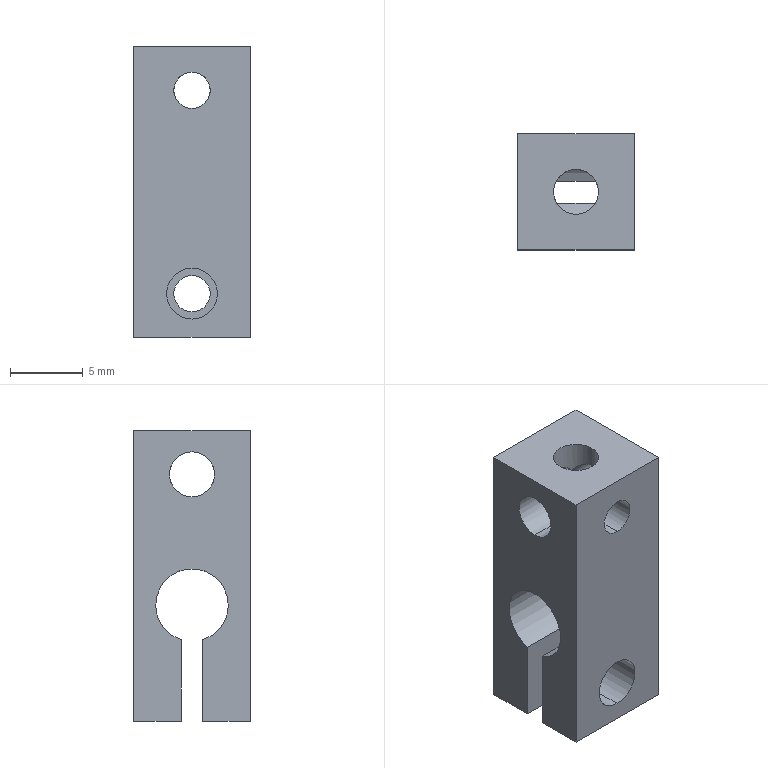Part | STEP file | 06-01-13 laser rotary plate A | 1 solid | 26 faces | box 8 x 8 x 20 mm | volume 871.542 mm3 | cylinder 17 | plane 9 | commonest cylinder face diameters 3.1 x8 2.5 x6 3.5 x2 5 x1
STEP:
#1=CARTESIAN_POINT('',(0.8839,-1.273,17.884));
#2=VERTEX_POINT('',#1);
#3=CARTESIAN_POINT('',(1.55,0.,18.55));
#4=VERTEX_POINT('',#3);
#5=CARTESIAN_POINT('',(0.8839,-1.273,17.884));
#6=CARTESIAN_POINT('',(1.31,-0.9777,18.31));
#7=CARTESIAN_POINT('',(1.55,-0.5184,18.55));
#8=CARTESIAN_POINT('',(1.55,0.,18.55));
#9=(BOUNDED_CURVE()B_SPLINE_CURVE(3,(#5,#6,#7,#8),.UNSPECIFIED.,.F.,.F.)B_SPLINE_CURVE_WITH_KNOTS((4,4),(2.178,3.142),.UNSPECIFIED.)CURVE()GEOMETRIC_REPRESENTATION_ITEM()RATIONAL_B_SPLINE_CURVE((1.,0.924,0.924,1.))REPRESENTATION_ITEM(''));
#10=EDGE_CURVE('',#2,#4,#9,.T.);
#11=ORIENTED_EDGE('',*,*,#10,.T.);
#12=CARTESIAN_POINT('',(4.,0.,18.55));
#13=VERTEX_POINT('',#12);
#14=CARTESIAN_POINT('',(4.,0.,18.55));
#15=DIRECTION('',(1.,0.,0.));
#16=VECTOR('',#15,1000.);
#17=LINE('',#14,#16);
#18=EDGE_CURVE('',#4,#13,#17,.T.);
#19=ORIENTED_EDGE('',*,*,#18,.T.);
#20=CARTESIAN_POINT('',(4.,0.,15.45));
#21=VERTEX_POINT('',#20);
#22=CARTESIAN_POINT('',(4.,0.,17.));
#23=DIRECTION('',(1.,0.,0.));
#24=DIRECTION('',(0.,0.,-1.));
#25=AXIS2_PLACEMENT_3D('',#22,#23,#24);
#26=CIRCLE('',#25,1.55);
#27=EDGE_CURVE('',#13,#21,#26,.T.);
#28=ORIENTED_EDGE('',*,*,#27,.T.);
#29=CARTESIAN_POINT('',(1.55,0.,15.45));
#30=VERTEX_POINT('',#29);
#31=CARTESIAN_POINT('',(4.,0.,15.45));
#32=DIRECTION('',(1.,0.,0.));
#33=VECTOR('',#32,1000.);
#34=LINE('',#31,#33);
#35=EDGE_CURVE('',#30,#21,#34,.T.);
#36=ORIENTED_EDGE('',*,*,#35,.F.);
#37=CARTESIAN_POINT('',(0.8839,-1.273,16.116));
#38=VERTEX_POINT('',#37);
#39=CARTESIAN_POINT('',(1.55,0.,15.45));
#40=CARTESIAN_POINT('',(1.55,-0.5184,15.45));
#41=CARTESIAN_POINT('',(1.31,-0.9777,15.69));
#42=CARTESIAN_POINT('',(0.8839,-1.273,16.116));
#43=(BOUNDED_CURVE()B_SPLINE_CURVE(3,(#39,#40,#41,#42),.UNSPECIFIED.,.F.,.F.)B_SPLINE_CURVE_WITH_KNOTS((4,4),(0.,0.964),.UNSPECIFIED.)CURVE()GEOMETRIC_REPRESENTATION_ITEM()RATIONAL_B_SPLINE_CURVE((1.,0.924,0.924,1.))REPRESENTATION_ITEM(''));
#44=EDGE_CURVE('',#30,#38,#43,.T.);
#45=ORIENTED_EDGE('',*,*,#44,.T.);
#46=CARTESIAN_POINT('',(0.8839,-1.273,17.884));
#47=CARTESIAN_POINT('',(0.9923,-1.349,17.775));
#48=CARTESIAN_POINT('',(1.083,-1.419,17.645));
#49=CARTESIAN_POINT('',(1.181,-1.495,17.418));
#50=CARTESIAN_POINT('',(1.206,-1.515,17.338));
#51=CARTESIAN_POINT('',(1.241,-1.543,17.173));
#52=CARTESIAN_POINT('',(1.25,-1.55,17.086));
#53=CARTESIAN_POINT('',(1.25,-1.55,16.83));
#54=CARTESIAN_POINT('',(1.214,-1.521,16.66));
#55=CARTESIAN_POINT('',(1.084,-1.419,16.357));
#56=CARTESIAN_POINT('',(0.9926,-1.349,16.225));
#57=CARTESIAN_POINT('',(0.8839,-1.273,16.116));
#58=B_SPLINE_CURVE_WITH_KNOTS('',3,(#46,#47,#48,#49,#50,#51,#52,#53,#54,#55,#56,#57),.UNSPECIFIED.,.F.,.F.,(4,2,2,2,2,4),(0.001052,0.001565,0.001821,0.002077,0.00259,0.003103),.UNSPECIFIED.);
#59=EDGE_CURVE('',#2,#38,#58,.T.);
#60=ORIENTED_EDGE('',*,*,#59,.F.);
#61=EDGE_LOOP('',(#11,#19,#28,#36,#45,#60));
#62=FACE_OUTER_BOUND('',#61,.T.);
#63=CARTESIAN_POINT('',(4.,0.,17.));
#64=DIRECTION('',(1.,0.,0.));
#65=DIRECTION('',(0.,0.,-1.));
#66=AXIS2_PLACEMENT_3D('',#63,#64,#65);
#67=CYLINDRICAL_SURFACE('',#66,1.55);
#68=ADVANCED_FACE('',(#62),#67,.F.);
#69=CARTESIAN_POINT('',(-4.,0.,18.55));
#70=VERTEX_POINT('',#69);
#71=CARTESIAN_POINT('',(-4.,0.,15.45));
#72=VERTEX_POINT('',#71);
#73=CARTESIAN_POINT('',(-4.,0.,17.));
#74=DIRECTION('',(1.,0.,0.));
#75=DIRECTION('',(0.,0.,-1.));
#76=AXIS2_PLACEMENT_3D('',#73,#74,#75);
#77=CIRCLE('',#76,1.55);
#78=EDGE_CURVE('',#70,#72,#77,.T.);
#79=ORIENTED_EDGE('',*,*,#78,.F.);
#80=CARTESIAN_POINT('',(-1.55,0.,18.55));
#81=VERTEX_POINT('',#80);
#82=CARTESIAN_POINT('',(4.,0.,18.55));
#83=DIRECTION('',(1.,0.,0.));
#84=VECTOR('',#83,1000.);
#85=LINE('',#82,#84);
#86=EDGE_CURVE('',#70,#81,#85,.T.);
#87=ORIENTED_EDGE('',*,*,#86,.T.);
#88=CARTESIAN_POINT('',(-0.8839,-1.273,17.884));
#89=VERTEX_POINT('',#88);
#90=CARTESIAN_POINT('',(-1.55,0.,18.55));
#91=CARTESIAN_POINT('',(-1.55,-0.5184,18.55));
#92=CARTESIAN_POINT('',(-1.31,-0.9777,18.31));
#93=CARTESIAN_POINT('',(-0.8839,-1.273,17.884));
#94=(BOUNDED_CURVE()B_SPLINE_CURVE(3,(#90,#91,#92,#93),.UNSPECIFIED.,.F.,.F.)B_SPLINE_CURVE_WITH_KNOTS((4,4),(3.142,4.106),.UNSPECIFIED.)CURVE()GEOMETRIC_REPRESENTATION_ITEM()RATIONAL_B_SPLINE_CURVE((1.,0.924,0.924,1.))REPRESENTATION_ITEM(''));
#95=EDGE_CURVE('',#81,#89,#94,.T.);
#96=ORIENTED_EDGE('',*,*,#95,.T.);
#97=CARTESIAN_POINT('',(-0.8839,-1.273,16.116));
#98=VERTEX_POINT('',#97);
#99=CARTESIAN_POINT('',(-0.8839,-1.273,16.116));
#100=CARTESIAN_POINT('',(-0.9934,-1.349,16.226));
#101=CARTESIAN_POINT('',(-1.082,-1.418,16.353));
#102=CARTESIAN_POINT('',(-1.181,-1.494,16.581));
#103=CARTESIAN_POINT('',(-1.206,-1.515,16.66));
#104=CARTESIAN_POINT('',(-1.241,-1.542,16.826));
#105=CARTESIAN_POINT('',(-1.25,-1.55,16.913));
#106=CARTESIAN_POINT('',(-1.25,-1.55,17.083));
#107=CARTESIAN_POINT('',(-1.241,-1.543,17.17));
#108=CARTESIAN_POINT('',(-1.207,-1.515,17.336));
#109=CARTESIAN_POINT('',(-1.182,-1.495,17.415));
#110=CARTESIAN_POINT('',(-1.084,-1.419,17.644));
#111=CARTESIAN_POINT('',(-0.9927,-1.349,17.775));
#112=CARTESIAN_POINT('',(-0.8839,-1.273,17.884));
#113=B_SPLINE_CURVE_WITH_KNOTS('',3,(#99,#100,#101,#102,#103,#104,#105,#106,#107,#108,#109,#110,#111,#112),.UNSPECIFIED.,.F.,.F.,(4,2,2,2,2,2,4),(0.005203,0.005716,0.005972,0.006228,0.006485,0.006741,0.007253),.UNSPECIFIED.);
#114=EDGE_CURVE('',#98,#89,#113,.T.);
#115=ORIENTED_EDGE('',*,*,#114,.F.);
#116=CARTESIAN_POINT('',(-1.55,0.,15.45));
#117=VERTEX_POINT('',#116);
#118=CARTESIAN_POINT('',(-0.8839,-1.273,16.116));
#119=CARTESIAN_POINT('',(-1.31,-0.9777,15.69));
#120=CARTESIAN_POINT('',(-1.55,-0.5184,15.45));
#121=CARTESIAN_POINT('',(-1.55,0.,15.45));
#122=(BOUNDED_CURVE()B_SPLINE_CURVE(3,(#118,#119,#120,#121),.UNSPECIFIED.,.F.,.F.)B_SPLINE_CURVE_WITH_KNOTS((4,4),(5.319,6.283),.UNSPECIFIED.)CURVE()GEOMETRIC_REPRESENTATION_ITEM()RATIONAL_B_SPLINE_CURVE((1.,0.924,0.924,1.))REPRESENTATION_ITEM(''));
#123=EDGE_CURVE('',#98,#117,#122,.T.);
#124=ORIENTED_EDGE('',*,*,#123,.T.);
#125=CARTESIAN_POINT('',(4.,0.,15.45));
#126=DIRECTION('',(1.,0.,0.));
#127=VECTOR('',#126,1000.);
#128=LINE('',#125,#127);
#129=EDGE_CURVE('',#72,#117,#128,.T.);
#130=ORIENTED_EDGE('',*,*,#129,.F.);
#131=EDGE_LOOP('',(#79,#87,#96,#115,#124,#130));
#132=FACE_OUTER_BOUND('',#131,.T.);
#133=CARTESIAN_POINT('',(4.,0.,17.));
#134=DIRECTION('',(1.,0.,0.));
#135=DIRECTION('',(0.,0.,-1.));
#136=AXIS2_PLACEMENT_3D('',#133,#134,#135);
#137=CYLINDRICAL_SURFACE('',#136,1.55);
#138=ADVANCED_FACE('',(#132),#137,.F.);
#139=CARTESIAN_POINT('',(0.,0.75,1.75));
#140=VERTEX_POINT('',#139);
#141=CARTESIAN_POINT('',(0.,0.75,4.25));
#142=VERTEX_POINT('',#141);
#143=CARTESIAN_POINT('',(0.,0.75,3.));
#144=DIRECTION('',(0.,1.,0.));
#145=DIRECTION('',(0.,0.,1.));
#146=AXIS2_PLACEMENT_3D('',#143,#144,#145);
#147=CIRCLE('',#146,1.25);
#148=EDGE_CURVE('',#140,#142,#147,.T.);
#149=ORIENTED_EDGE('',*,*,#148,.F.);
#150=CARTESIAN_POINT('',(0.,4.,1.75));
#151=VERTEX_POINT('',#150);
#152=CARTESIAN_POINT('',(0.,4.,1.75));
#153=DIRECTION('',(0.,1.,0.));
#154=VECTOR('',#153,1000.);
#155=LINE('',#152,#154);
#156=EDGE_CURVE('',#140,#151,#155,.T.);
#157=ORIENTED_EDGE('',*,*,#156,.T.);
#158=CARTESIAN_POINT('',(0.,4.,4.25));
#159=VERTEX_POINT('',#158);
#160=CARTESIAN_POINT('',(0.,4.,3.));
#161=DIRECTION('',(0.,1.,0.));
#162=DIRECTION('',(0.,0.,1.));
#163=AXIS2_PLACEMENT_3D('',#160,#161,#162);
#164=CIRCLE('',#163,1.25);
#165=EDGE_CURVE('',#151,#159,#164,.T.);
#166=ORIENTED_EDGE('',*,*,#165,.T.);
#167=CARTESIAN_POINT('',(0.,4.,4.25));
#168=DIRECTION('',(0.,1.,0.));
#169=VECTOR('',#168,1000.);
#170=LINE('',#167,#169);
#171=EDGE_CURVE('',#142,#159,#170,.T.);
#172=ORIENTED_EDGE('',*,*,#171,.F.);
#173=EDGE_LOOP('',(#149,#157,#166,#172));
#174=FACE_OUTER_BOUND('',#173,.T.);
#175=CARTESIAN_POINT('',(0.,4.,3.));
#176=DIRECTION('',(0.,1.,0.));
#177=DIRECTION('',(0.,0.,1.));
#178=AXIS2_PLACEMENT_3D('',#175,#176,#177);
#179=CYLINDRICAL_SURFACE('',#178,1.25);
#180=ADVANCED_FACE('',(#174),#179,.F.);
#181=CARTESIAN_POINT('',(0.,-4.,15.75));
#182=VERTEX_POINT('',#181);
#183=CARTESIAN_POINT('',(0.,-4.,18.25));
#184=VERTEX_POINT('',#183);
#185=CARTESIAN_POINT('',(0.,-4.,17.));
#186=DIRECTION('',(0.,1.,0.));
#187=DIRECTION('',(0.,0.,1.));
#188=AXIS2_PLACEMENT_3D('',#185,#186,#187);
#189=CIRCLE('',#188,1.25);
#190=EDGE_CURVE('',#182,#184,#189,.T.);
#191=ORIENTED_EDGE('',*,*,#190,.F.);
#192=CARTESIAN_POINT('',(0.,-1.55,15.75));
#193=VERTEX_POINT('',#192);
#194=CARTESIAN_POINT('',(0.,4.,15.75));
#195=DIRECTION('',(0.,1.,0.));
#196=VECTOR('',#195,1000.);
#197=LINE('',#194,#196);
#198=EDGE_CURVE('',#182,#193,#197,.T.);
#199=ORIENTED_EDGE('',*,*,#198,.T.);
#200=CARTESIAN_POINT('',(0.,-1.55,15.75));
#201=CARTESIAN_POINT('',(-0.1704,-1.55,15.75));
#202=CARTESIAN_POINT('',(-0.3419,-1.52,15.786));
#203=CARTESIAN_POINT('',(-0.6439,-1.419,15.916));
#204=CARTESIAN_POINT('',(-0.7753,-1.349,16.008));
#205=CARTESIAN_POINT('',(-0.8839,-1.273,16.116));
#206=B_SPLINE_CURVE_WITH_KNOTS('',3,(#200,#201,#202,#203,#204,#205),.UNSPECIFIED.,.F.,.F.,(4,2,4),(0.004146,0.004656,0.005166),.UNSPECIFIED.);
#207=EDGE_CURVE('',#193,#98,#206,.T.);
#208=ORIENTED_EDGE('',*,*,#207,.T.);
#209=ORIENTED_EDGE('',*,*,#114,.T.);
#210=CARTESIAN_POINT('',(0.,-1.55,18.25));
#211=VERTEX_POINT('',#210);
#212=CARTESIAN_POINT('',(-0.8839,-1.273,17.884));
#213=CARTESIAN_POINT('',(-0.7745,-1.349,17.993));
#214=CARTESIAN_POINT('',(-0.6461,-1.418,18.083));
#215=CARTESIAN_POINT('',(-0.4186,-1.495,18.181));
#216=CARTESIAN_POINT('',(-0.3394,-1.515,18.206));
#217=CARTESIAN_POINT('',(-0.1734,-1.543,18.241));
#218=CARTESIAN_POINT('',(-0.08647,-1.55,18.25));
#219=CARTESIAN_POINT('',(0.,-1.55,18.25));
#220=B_SPLINE_CURVE_WITH_KNOTS('',3,(#212,#213,#214,#215,#216,#217,#218,#219),.UNSPECIFIED.,.F.,.F.,(4,2,2,4),(0.007258,0.007768,0.008024,0.008279),.UNSPECIFIED.);
#221=EDGE_CURVE('',#89,#211,#220,.T.);
#222=ORIENTED_EDGE('',*,*,#221,.T.);
#223=CARTESIAN_POINT('',(0.,4.,18.25));
#224=DIRECTION('',(0.,1.,0.));
#225=VECTOR('',#224,1000.);
#226=LINE('',#223,#225);
#227=EDGE_CURVE('',#184,#211,#226,.T.);
#228=ORIENTED_EDGE('',*,*,#227,.F.);
#229=EDGE_LOOP('',(#191,#199,#208,#209,#222,#228));
#230=FACE_OUTER_BOUND('',#229,.T.);
#231=CARTESIAN_POINT('',(0.,4.,17.));
#232=DIRECTION('',(0.,1.,0.));
#233=DIRECTION('',(0.,0.,1.));
#234=AXIS2_PLACEMENT_3D('',#231,#232,#233);
#235=CYLINDRICAL_SURFACE('',#234,1.25);
#236=ADVANCED_FACE('',(#230),#235,.F.);
#237=CARTESIAN_POINT('',(-0.8839,1.273,16.116));
#238=VERTEX_POINT('',#237);
#239=CARTESIAN_POINT('',(0.,1.55,15.75));
#240=VERTEX_POINT('',#239);
#241=CARTESIAN_POINT('',(-0.8839,1.273,16.116));
#242=CARTESIAN_POINT('',(-0.8293,1.311,16.062));
#243=CARTESIAN_POINT('',(-0.77,1.347,16.012));
#244=CARTESIAN_POINT('',(-0.6402,1.414,15.923));
#245=CARTESIAN_POINT('',(-0.5688,1.444,15.884));
#246=CARTESIAN_POINT('',(-0.3422,1.52,15.787));
#247=CARTESIAN_POINT('',(-0.1711,1.55,15.75));
#248=CARTESIAN_POINT('',(0.,1.55,15.75));
#249=B_SPLINE_CURVE_WITH_KNOTS('',3,(#241,#242,#243,#244,#245,#246,#247,#248),.UNSPECIFIED.,.F.,.F.,(4,2,2,4),(0.003121,0.003377,0.003633,0.004146),.UNSPECIFIED.);
#250=EDGE_CURVE('',#238,#240,#249,.T.);
#251=ORIENTED_EDGE('',*,*,#250,.T.);
#252=CARTESIAN_POINT('',(0.,4.,15.75));
#253=VERTEX_POINT('',#252);
#254=CARTESIAN_POINT('',(0.,4.,15.75));
#255=DIRECTION('',(0.,1.,0.));
#256=VECTOR('',#255,1000.);
#257=LINE('',#254,#256);
#258=EDGE_CURVE('',#240,#253,#257,.T.);
#259=ORIENTED_EDGE('',*,*,#258,.T.);
#260=CARTESIAN_POINT('',(0.,4.,18.25));
#261=VERTEX_POINT('',#260);
#262=CARTESIAN_POINT('',(0.,4.,17.));
#263=DIRECTION('',(0.,1.,0.));
#264=DIRECTION('',(0.,0.,1.));
#265=AXIS2_PLACEMENT_3D('',#262,#263,#264);
#266=CIRCLE('',#265,1.25);
#267=EDGE_CURVE('',#253,#261,#266,.T.);
#268=ORIENTED_EDGE('',*,*,#267,.T.);
#269=CARTESIAN_POINT('',(0.,1.55,18.25));
#270=VERTEX_POINT('',#269);
#271=CARTESIAN_POINT('',(0.,4.,18.25));
#272=DIRECTION('',(0.,1.,0.));
#273=VECTOR('',#272,1000.);
#274=LINE('',#271,#273);
#275=EDGE_CURVE('',#270,#261,#274,.T.);
#276=ORIENTED_EDGE('',*,*,#275,.F.);
#277=CARTESIAN_POINT('',(-0.8839,1.273,17.884));
#278=VERTEX_POINT('',#277);
#279=CARTESIAN_POINT('',(0.,1.55,18.25));
#280=CARTESIAN_POINT('',(-0.08678,1.55,18.25));
#281=CARTESIAN_POINT('',(-0.1714,1.543,18.241));
#282=CARTESIAN_POINT('',(-0.3369,1.515,18.207));
#283=CARTESIAN_POINT('',(-0.4179,1.495,18.181));
#284=CARTESIAN_POINT('',(-0.6435,1.419,18.084));
#285=CARTESIAN_POINT('',(-0.7755,1.349,17.992));
#286=CARTESIAN_POINT('',(-0.8839,1.273,17.884));
#287=B_SPLINE_CURVE_WITH_KNOTS('',3,(#279,#280,#281,#282,#283,#284,#285,#286),.UNSPECIFIED.,.F.,.F.,(4,2,2,4),(0.,0.000256,0.0005121,0.001024),.UNSPECIFIED.);
#288=EDGE_CURVE('',#270,#278,#287,.T.);
#289=ORIENTED_EDGE('',*,*,#288,.T.);
#290=CARTESIAN_POINT('',(-0.8839,1.273,17.884));
#291=CARTESIAN_POINT('',(-0.9923,1.349,17.775));
#292=CARTESIAN_POINT('',(-1.083,1.419,17.645));
#293=CARTESIAN_POINT('',(-1.181,1.495,17.418));
#294=CARTESIAN_POINT('',(-1.206,1.515,17.338));
#295=CARTESIAN_POINT('',(-1.241,1.543,17.173));
#296=CARTESIAN_POINT('',(-1.25,1.55,17.086));
#297=CARTESIAN_POINT('',(-1.25,1.55,16.83));
#298=CARTESIAN_POINT('',(-1.214,1.521,16.66));
#299=CARTESIAN_POINT('',(-1.084,1.419,16.357));
#300=CARTESIAN_POINT('',(-0.9926,1.349,16.225));
#301=CARTESIAN_POINT('',(-0.8839,1.273,16.116));
#302=B_SPLINE_CURVE_WITH_KNOTS('',3,(#290,#291,#292,#293,#294,#295,#296,#297,#298,#299,#300,#301),.UNSPECIFIED.,.F.,.F.,(4,2,2,2,2,4),(0.001052,0.001565,0.001821,0.002077,0.00259,0.003103),.UNSPECIFIED.);
#303=EDGE_CURVE('',#278,#238,#302,.T.);
#304=ORIENTED_EDGE('',*,*,#303,.T.);
#305=EDGE_LOOP('',(#251,#259,#268,#276,#289,#304));
#306=FACE_OUTER_BOUND('',#305,.T.);
#307=CARTESIAN_POINT('',(0.,4.,17.));
#308=DIRECTION('',(0.,1.,0.));
#309=DIRECTION('',(0.,0.,1.));
#310=AXIS2_PLACEMENT_3D('',#307,#308,#309);
#311=CYLINDRICAL_SURFACE('',#310,1.25);
#312=ADVANCED_FACE('',(#306),#311,.F.);
#313=CARTESIAN_POINT('',(0.,-0.75,4.75));
#314=VERTEX_POINT('',#313);
#315=CARTESIAN_POINT('',(0.,-0.75,1.25));
#316=VERTEX_POINT('',#315);
#317=CARTESIAN_POINT('',(0.,-0.75,3.));
#318=DIRECTION('',(0.,-1.,0.));
#319=DIRECTION('',(0.,0.,-1.));
#320=AXIS2_PLACEMENT_3D('',#317,#318,#319);
#321=CIRCLE('',#320,1.75);
#322=EDGE_CURVE('',#314,#316,#321,.T.);
#323=ORIENTED_EDGE('',*,*,#322,.F.);
#324=CARTESIAN_POINT('',(0.,-4.,4.75));
#325=VERTEX_POINT('',#324);
#326=CARTESIAN_POINT('',(0.,0.,4.75));
#327=DIRECTION('',(0.,-1.,0.));
#328=VECTOR('',#327,1000.);
#329=LINE('',#326,#328);
#330=EDGE_CURVE('',#314,#325,#329,.T.);
#331=ORIENTED_EDGE('',*,*,#330,.T.);
#332=CARTESIAN_POINT('',(0.,-4.,1.25));
#333=VERTEX_POINT('',#332);
#334=CARTESIAN_POINT('',(0.,-4.,3.));
#335=DIRECTION('',(0.,-1.,0.));
#336=DIRECTION('',(0.,0.,-1.));
#337=AXIS2_PLACEMENT_3D('',#334,#335,#336);
#338=CIRCLE('',#337,1.75);
#339=EDGE_CURVE('',#325,#333,#338,.T.);
#340=ORIENTED_EDGE('',*,*,#339,.T.);
#341=CARTESIAN_POINT('',(0.,0.,1.25));
#342=DIRECTION('',(0.,-1.,0.));
#343=VECTOR('',#342,1000.);
#344=LINE('',#341,#343);
#345=EDGE_CURVE('',#316,#333,#344,.T.);
#346=ORIENTED_EDGE('',*,*,#345,.F.);
#347=EDGE_LOOP('',(#323,#331,#340,#346));
#348=FACE_OUTER_BOUND('',#347,.T.);
#349=CARTESIAN_POINT('',(0.,0.,3.));
#350=DIRECTION('',(0.,-1.,0.));
#351=DIRECTION('',(0.,0.,-1.));
#352=AXIS2_PLACEMENT_3D('',#349,#350,#351);
#353=CYLINDRICAL_SURFACE('',#352,1.75);
#354=ADVANCED_FACE('',(#348),#353,.F.);
#355=ORIENTED_EDGE('',*,*,#44,.F.);
#356=CARTESIAN_POINT('',(1.55,0.,10.5));
#357=VERTEX_POINT('',#356);
#358=CARTESIAN_POINT('',(1.55,0.,20.));
#359=DIRECTION('',(0.,0.,-1.));
#360=VECTOR('',#359,1000.);
#361=LINE('',#358,#360);
#362=EDGE_CURVE('',#30,#357,#361,.T.);
#363=ORIENTED_EDGE('',*,*,#362,.T.);
#364=CARTESIAN_POINT('',(-1.55,0.,10.5));
#365=VERTEX_POINT('',#364);
#366=CARTESIAN_POINT('',(-1.55,0.,10.5));
#367=CARTESIAN_POINT('',(-1.55,-0.1055,10.5));
#368=CARTESIAN_POINT('',(-1.539,-0.2087,10.493));
#369=CARTESIAN_POINT('',(-1.498,-0.411,10.468));
#370=CARTESIAN_POINT('',(-1.467,-0.5109,10.449));
#371=CARTESIAN_POINT('',(-1.348,-0.7915,10.379));
#372=CARTESIAN_POINT('',(-1.233,-0.9593,10.314));
#373=CARTESIAN_POINT('',(-1.024,-1.168,10.212));
#374=CARTESIAN_POINT('',(-0.9469,-1.231,10.177));
#375=CARTESIAN_POINT('',(-0.7828,-1.341,10.111));
#376=CARTESIAN_POINT('',(-0.6959,-1.389,10.079));
#377=CARTESIAN_POINT('',(-0.4186,-1.506,9.998));
#378=CARTESIAN_POINT('',(-0.2106,-1.55,9.962));
#379=CARTESIAN_POINT('',(0.1045,-1.55,9.961));
#380=CARTESIAN_POINT('',(0.2076,-1.54,9.97));
#381=CARTESIAN_POINT('',(0.4105,-1.498,10.001));
#382=CARTESIAN_POINT('',(0.5091,-1.467,10.025));
#383=CARTESIAN_POINT('',(0.6949,-1.389,10.079));
#384=CARTESIAN_POINT('',(0.7838,-1.341,10.111));
#385=CARTESIAN_POINT('',(0.9481,-1.23,10.177));
#386=CARTESIAN_POINT('',(1.024,-1.168,10.212));
#387=CARTESIAN_POINT('',(1.235,-0.9576,10.315));
#388=CARTESIAN_POINT('',(1.347,-0.7932,10.379));
#389=CARTESIAN_POINT('',(1.468,-0.5092,10.45));
#390=CARTESIAN_POINT('',(1.498,-0.4114,10.468));
#391=CARTESIAN_POINT('',(1.539,-0.21,10.493));
#392=CARTESIAN_POINT('',(1.55,-0.1048,10.5));
#393=CARTESIAN_POINT('',(1.55,0.,10.5));
#394=B_SPLINE_CURVE_WITH_KNOTS('',3,(#366,#367,#368,#369,#370,#371,#372,#373,#374,#375,#376,#377,#378,#379,#380,#381,#382,#383,#384,#385,#386,#387,#388,#389,#390,#391,#392,#393),.UNSPECIFIED.,.F.,.F.,(4,2,2,2,2,2,2,2,2,2,2,2,2,4),(0.,0.0003115,0.0006229,0.001246,0.001557,0.001869,0.002492,0.002803,0.003115,0.003426,0.003737,0.00436,0.004672,0.004983),.UNSPECIFIED.);
#395=EDGE_CURVE('',#365,#357,#394,.T.);
#396=ORIENTED_EDGE('',*,*,#395,.F.);
#397=CARTESIAN_POINT('',(-1.55,0.,20.));
#398=DIRECTION('',(0.,0.,-1.));
#399=VECTOR('',#398,1000.);
#400=LINE('',#397,#399);
#401=EDGE_CURVE('',#117,#365,#400,.T.);
#402=ORIENTED_EDGE('',*,*,#401,.F.);
#403=ORIENTED_EDGE('',*,*,#123,.F.);
#404=ORIENTED_EDGE('',*,*,#207,.F.);
#405=CARTESIAN_POINT('',(0.8839,-1.273,16.116));
#406=CARTESIAN_POINT('',(0.8293,-1.311,16.062));
#407=CARTESIAN_POINT('',(0.77,-1.347,16.012));
#408=CARTESIAN_POINT('',(0.6402,-1.414,15.923));
#409=CARTESIAN_POINT('',(0.5688,-1.444,15.884));
#410=CARTESIAN_POINT('',(0.3422,-1.52,15.787));
#411=CARTESIAN_POINT('',(0.1711,-1.55,15.75));
#412=CARTESIAN_POINT('',(0.,-1.55,15.75));
#413=B_SPLINE_CURVE_WITH_KNOTS('',3,(#405,#406,#407,#408,#409,#410,#411,#412),.UNSPECIFIED.,.F.,.F.,(4,2,2,4),(0.003121,0.003377,0.003633,0.004146),.UNSPECIFIED.);
#414=EDGE_CURVE('',#38,#193,#413,.T.);
#415=ORIENTED_EDGE('',*,*,#414,.F.);
#416=EDGE_LOOP('',(#355,#363,#396,#402,#403,#404,#415));
#417=FACE_OUTER_BOUND('',#416,.T.);
#418=CARTESIAN_POINT('',(0.,0.,20.));
#419=DIRECTION('',(0.,0.,-1.));
#420=DIRECTION('',(-1.,0.,0.));
#421=AXIS2_PLACEMENT_3D('',#418,#419,#420);
#422=CYLINDRICAL_SURFACE('',#421,1.55);
#423=ADVANCED_FACE('',(#417),#422,.F.);
#424=CARTESIAN_POINT('',(-1.55,0.,20.));
#425=VERTEX_POINT('',#424);
#426=CARTESIAN_POINT('',(1.55,0.,20.));
#427=VERTEX_POINT('',#426);
#428=CARTESIAN_POINT('',(0.,0.,20.));
#429=DIRECTION('',(0.,0.,1.));
#430=DIRECTION('',(1.,0.,0.));
#431=AXIS2_PLACEMENT_3D('',#428,#429,#430);
#432=CIRCLE('',#431,1.55);
#433=EDGE_CURVE('',#425,#427,#432,.T.);
#434=ORIENTED_EDGE('',*,*,#433,.T.);
#435=CARTESIAN_POINT('',(1.55,0.,20.));
#436=DIRECTION('',(0.,0.,-1.));
#437=VECTOR('',#436,1000.);
#438=LINE('',#435,#437);
#439=EDGE_CURVE('',#427,#4,#438,.T.);
#440=ORIENTED_EDGE('',*,*,#439,.T.);
#441=ORIENTED_EDGE('',*,*,#10,.F.);
#442=CARTESIAN_POINT('',(0.,-1.55,18.25));
#443=CARTESIAN_POINT('',(0.08678,-1.55,18.25));
#444=CARTESIAN_POINT('',(0.1714,-1.543,18.241));
#445=CARTESIAN_POINT('',(0.3369,-1.515,18.207));
#446=CARTESIAN_POINT('',(0.4179,-1.495,18.181));
#447=CARTESIAN_POINT('',(0.6435,-1.419,18.084));
#448=CARTESIAN_POINT('',(0.7755,-1.349,17.992));
#449=CARTESIAN_POINT('',(0.8839,-1.273,17.884));
#450=B_SPLINE_CURVE_WITH_KNOTS('',3,(#442,#443,#444,#445,#446,#447,#448,#449),.UNSPECIFIED.,.F.,.F.,(4,2,2,4),(0.,0.000256,0.0005121,0.001024),.UNSPECIFIED.);
#451=EDGE_CURVE('',#211,#2,#450,.T.);
#452=ORIENTED_EDGE('',*,*,#451,.F.);
#453=ORIENTED_EDGE('',*,*,#221,.F.);
#454=ORIENTED_EDGE('',*,*,#95,.F.);
#455=CARTESIAN_POINT('',(-1.55,0.,20.));
#456=DIRECTION('',(0.,0.,-1.));
#457=VECTOR('',#456,1000.);
#458=LINE('',#455,#457);
#459=EDGE_CURVE('',#425,#81,#458,.T.);
#460=ORIENTED_EDGE('',*,*,#459,.F.);
#461=EDGE_LOOP('',(#434,#440,#441,#452,#453,#454,#460));
#462=FACE_OUTER_BOUND('',#461,.T.);
#463=CARTESIAN_POINT('',(0.,0.,20.));
#464=DIRECTION('',(0.,0.,-1.));
#465=DIRECTION('',(-1.,0.,0.));
#466=AXIS2_PLACEMENT_3D('',#463,#464,#465);
#467=CYLINDRICAL_SURFACE('',#466,1.55);
#468=ADVANCED_FACE('',(#462),#467,.F.);
#469=ORIENTED_EDGE('',*,*,#439,.F.);
#470=CARTESIAN_POINT('',(0.,0.,20.));
#471=DIRECTION('',(0.,0.,1.));
#472=DIRECTION('',(1.,0.,0.));
#473=AXIS2_PLACEMENT_3D('',#470,#471,#472);
#474=CIRCLE('',#473,1.55);
#475=EDGE_CURVE('',#427,#425,#474,.T.);
#476=ORIENTED_EDGE('',*,*,#475,.T.);
#477=ORIENTED_EDGE('',*,*,#459,.T.);
#478=CARTESIAN_POINT('',(-0.8839,1.273,17.884));
#479=CARTESIAN_POINT('',(-1.31,0.9777,18.31));
#480=CARTESIAN_POINT('',(-1.55,0.5184,18.55));
#481=CARTESIAN_POINT('',(-1.55,0.,18.55));
#482=(BOUNDED_CURVE()B_SPLINE_CURVE(3,(#478,#479,#480,#481),.UNSPECIFIED.,.F.,.F.)B_SPLINE_CURVE_WITH_KNOTS((4,4),(2.178,3.142),.UNSPECIFIED.)CURVE()GEOMETRIC_REPRESENTATION_ITEM()RATIONAL_B_SPLINE_CURVE((1.,0.924,0.924,1.))REPRESENTATION_ITEM(''));
#483=EDGE_CURVE('',#278,#81,#482,.T.);
#484=ORIENTED_EDGE('',*,*,#483,.F.);
#485=ORIENTED_EDGE('',*,*,#288,.F.);
#486=CARTESIAN_POINT('',(0.8839,1.273,17.884));
#487=VERTEX_POINT('',#486);
#488=CARTESIAN_POINT('',(0.8839,1.273,17.884));
#489=CARTESIAN_POINT('',(0.7745,1.349,17.993));
#490=CARTESIAN_POINT('',(0.6461,1.418,18.083));
#491=CARTESIAN_POINT('',(0.4186,1.495,18.181));
#492=CARTESIAN_POINT('',(0.3394,1.515,18.206));
#493=CARTESIAN_POINT('',(0.1734,1.543,18.241));
#494=CARTESIAN_POINT('',(0.08647,1.55,18.25));
#495=CARTESIAN_POINT('',(0.,1.55,18.25));
#496=B_SPLINE_CURVE_WITH_KNOTS('',3,(#488,#489,#490,#491,#492,#493,#494,#495),.UNSPECIFIED.,.F.,.F.,(4,2,2,4),(0.007258,0.007768,0.008024,0.008279),.UNSPECIFIED.);
#497=EDGE_CURVE('',#487,#270,#496,.T.);
#498=ORIENTED_EDGE('',*,*,#497,.F.);
#499=CARTESIAN_POINT('',(1.55,0.,18.55));
#500=CARTESIAN_POINT('',(1.55,0.5184,18.55));
#501=CARTESIAN_POINT('',(1.31,0.9777,18.31));
#502=CARTESIAN_POINT('',(0.8839,1.273,17.884));
#503=(BOUNDED_CURVE()B_SPLINE_CURVE(3,(#499,#500,#501,#502),.UNSPECIFIED.,.F.,.F.)B_SPLINE_CURVE_WITH_KNOTS((4,4),(3.142,4.106),.UNSPECIFIED.)CURVE()GEOMETRIC_REPRESENTATION_ITEM()RATIONAL_B_SPLINE_CURVE((1.,0.924,0.924,1.))REPRESENTATION_ITEM(''));
#504=EDGE_CURVE('',#4,#487,#503,.T.);
#505=ORIENTED_EDGE('',*,*,#504,.F.);
#506=EDGE_LOOP('',(#469,#476,#477,#484,#485,#498,#505));
#507=FACE_OUTER_BOUND('',#506,.T.);
#508=CARTESIAN_POINT('',(0.,0.,20.));
#509=DIRECTION('',(0.,0.,-1.));
#510=DIRECTION('',(-1.,0.,0.));
#511=AXIS2_PLACEMENT_3D('',#508,#509,#510);
#512=CYLINDRICAL_SURFACE('',#511,1.55);
#513=ADVANCED_FACE('',(#507),#512,.F.);
#514=CARTESIAN_POINT('',(4.,0.75,0.));
#515=VERTEX_POINT('',#514);
#516=CARTESIAN_POINT('',(4.,4.,0.));
#517=VERTEX_POINT('',#516);
#518=CARTESIAN_POINT('',(4.,4.,0.));
#519=DIRECTION('',(0.,1.,0.));
#520=VECTOR('',#519,1000.);
#521=LINE('',#518,#520);
#522=EDGE_CURVE('',#515,#517,#521,.T.);
#523=ORIENTED_EDGE('',*,*,#522,.F.);
#524=CARTESIAN_POINT('',(-4.,0.75,0.));
#525=VERTEX_POINT('',#524);
#526=CARTESIAN_POINT('',(4.,0.75,0.));
#527=DIRECTION('',(-1.,0.,0.));
#528=VECTOR('',#527,1000.);
#529=LINE('',#526,#528);
#530=EDGE_CURVE('',#515,#525,#529,.T.);
#531=ORIENTED_EDGE('',*,*,#530,.T.);
#532=CARTESIAN_POINT('',(-4.,4.,0.));
#533=VERTEX_POINT('',#532);
#534=CARTESIAN_POINT('',(-4.,4.,0.));
#535=DIRECTION('',(0.,-1.,0.));
#536=VECTOR('',#535,1000.);
#537=LINE('',#534,#536);
#538=EDGE_CURVE('',#533,#525,#537,.T.);
#539=ORIENTED_EDGE('',*,*,#538,.F.);
#540=CARTESIAN_POINT('',(-4.,4.,0.));
#541=DIRECTION('',(-1.,0.,0.));
#542=VECTOR('',#541,1000.);
#543=LINE('',#540,#542);
#544=EDGE_CURVE('',#517,#533,#543,.T.);
#545=ORIENTED_EDGE('',*,*,#544,.F.);
#546=EDGE_LOOP('',(#523,#531,#539,#545));
#547=FACE_OUTER_BOUND('',#546,.T.);
#548=CARTESIAN_POINT('',(4.,-4.,0.));
#549=DIRECTION('',(0.,0.,1.));
#550=DIRECTION('',(1.,0.,0.));
#551=AXIS2_PLACEMENT_3D('',#548,#549,#550);
#552=PLANE('',#551);
#553=ADVANCED_FACE('',(#547),#552,.F.);
#554=ORIENTED_EDGE('',*,*,#362,.F.);
#555=CARTESIAN_POINT('',(0.8839,1.273,16.116));
#556=VERTEX_POINT('',#555);
#557=CARTESIAN_POINT('',(0.8839,1.273,16.116));
#558=CARTESIAN_POINT('',(1.31,0.9777,15.69));
#559=CARTESIAN_POINT('',(1.55,0.5184,15.45));
#560=CARTESIAN_POINT('',(1.55,0.,15.45));
#561=(BOUNDED_CURVE()B_SPLINE_CURVE(3,(#557,#558,#559,#560),.UNSPECIFIED.,.F.,.F.)B_SPLINE_CURVE_WITH_KNOTS((4,4),(5.319,6.283),.UNSPECIFIED.)CURVE()GEOMETRIC_REPRESENTATION_ITEM()RATIONAL_B_SPLINE_CURVE((1.,0.924,0.924,1.))REPRESENTATION_ITEM(''));
#562=EDGE_CURVE('',#556,#30,#561,.T.);
#563=ORIENTED_EDGE('',*,*,#562,.F.);
#564=CARTESIAN_POINT('',(0.,1.55,15.75));
#565=CARTESIAN_POINT('',(0.1704,1.55,15.75));
#566=CARTESIAN_POINT('',(0.3419,1.52,15.786));
#567=CARTESIAN_POINT('',(0.6439,1.419,15.916));
#568=CARTESIAN_POINT('',(0.7753,1.349,16.008));
#569=CARTESIAN_POINT('',(0.8839,1.273,16.116));
#570=B_SPLINE_CURVE_WITH_KNOTS('',3,(#564,#565,#566,#567,#568,#569),.UNSPECIFIED.,.F.,.F.,(4,2,4),(0.004146,0.004656,0.005166),.UNSPECIFIED.);
#571=EDGE_CURVE('',#240,#556,#570,.T.);
#572=ORIENTED_EDGE('',*,*,#571,.F.);
#573=ORIENTED_EDGE('',*,*,#250,.F.);
#574=CARTESIAN_POINT('',(-1.55,0.,15.45));
#575=CARTESIAN_POINT('',(-1.55,0.5184,15.45));
#576=CARTESIAN_POINT('',(-1.31,0.9777,15.69));
#577=CARTESIAN_POINT('',(-0.8839,1.273,16.116));
#578=(BOUNDED_CURVE()B_SPLINE_CURVE(3,(#574,#575,#576,#577),.UNSPECIFIED.,.F.,.F.)B_SPLINE_CURVE_WITH_KNOTS((4,4),(0.,0.964),.UNSPECIFIED.)CURVE()GEOMETRIC_REPRESENTATION_ITEM()RATIONAL_B_SPLINE_CURVE((1.,0.924,0.924,1.))REPRESENTATION_ITEM(''));
#579=EDGE_CURVE('',#117,#238,#578,.T.);
#580=ORIENTED_EDGE('',*,*,#579,.F.);
#581=ORIENTED_EDGE('',*,*,#401,.T.);
#582=CARTESIAN_POINT('',(1.55,0.,10.5));
#583=CARTESIAN_POINT('',(1.55,0.1046,10.5));
#584=CARTESIAN_POINT('',(1.54,0.2077,10.493));
#585=CARTESIAN_POINT('',(1.498,0.411,10.468));
#586=CARTESIAN_POINT('',(1.467,0.5104,10.449));
#587=CARTESIAN_POINT('',(1.388,0.6973,10.403));
#588=CARTESIAN_POINT('',(1.339,0.7869,10.375));
#589=CARTESIAN_POINT('',(1.227,0.9523,10.313));
#590=CARTESIAN_POINT('',(1.164,1.028,10.28));
#591=CARTESIAN_POINT('',(0.9539,1.238,10.178));
#592=CARTESIAN_POINT('',(0.7901,1.349,10.107));
#593=CARTESIAN_POINT('',(0.5097,1.467,10.025));
#594=CARTESIAN_POINT('',(0.4121,1.498,10.002));
#595=CARTESIAN_POINT('',(0.2104,1.539,9.97));
#596=CARTESIAN_POINT('',(0.1047,1.55,9.962));
#597=CARTESIAN_POINT('',(-0.2072,1.55,9.961));
#598=CARTESIAN_POINT('',(-0.4149,1.507,9.997));
#599=CARTESIAN_POINT('',(-0.7877,1.35,10.106));
#600=CARTESIAN_POINT('',(-0.9541,1.237,10.178));
#601=CARTESIAN_POINT('',(-1.164,1.028,10.28));
#602=CARTESIAN_POINT('',(-1.227,0.9522,10.313));
#603=CARTESIAN_POINT('',(-1.339,0.7876,10.374));
#604=CARTESIAN_POINT('',(-1.388,0.6977,10.403));
#605=CARTESIAN_POINT('',(-1.467,0.5109,10.449));
#606=CARTESIAN_POINT('',(-1.497,0.4138,10.468));
#607=CARTESIAN_POINT('',(-1.539,0.2114,10.493));
#608=CARTESIAN_POINT('',(-1.55,0.1052,10.5));
#609=CARTESIAN_POINT('',(-1.55,0.,10.5));
#610=B_SPLINE_CURVE_WITH_KNOTS('',3,(#582,#583,#584,#585,#586,#587,#588,#589,#590,#591,#592,#593,#594,#595,#596,#597,#598,#599,#600,#601,#602,#603,#604,#605,#606,#607,#608,#609),.UNSPECIFIED.,.F.,.F.,(4,2,2,2,2,2,2,2,2,2,2,2,2,4),(0.004983,0.005294,0.005605,0.005916,0.006226,0.006848,0.007159,0.007469,0.008091,0.008712,0.009023,0.009334,0.009645,0.009956),.UNSPECIFIED.);
#611=EDGE_CURVE('',#357,#365,#610,.T.);
#612=ORIENTED_EDGE('',*,*,#611,.F.);
#613=EDGE_LOOP('',(#554,#563,#572,#573,#580,#581,#612));
#614=FACE_OUTER_BOUND('',#613,.T.);
#615=CARTESIAN_POINT('',(0.,0.,20.));
#616=DIRECTION('',(0.,0.,-1.));
#617=DIRECTION('',(-1.,0.,0.));
#618=AXIS2_PLACEMENT_3D('',#615,#616,#617);
#619=CYLINDRICAL_SURFACE('',#618,1.55);
#620=ADVANCED_FACE('',(#614),#619,.F.);
#621=CARTESIAN_POINT('',(4.,-4.,20.));
#622=VERTEX_POINT('',#621);
#623=CARTESIAN_POINT('',(4.,4.,20.));
#624=VERTEX_POINT('',#623);
#625=CARTESIAN_POINT('',(4.,4.,20.));
#626=DIRECTION('',(0.,1.,0.));
#627=VECTOR('',#626,1000.);
#628=LINE('',#625,#627);
#629=EDGE_CURVE('',#622,#624,#628,.T.);
#630=ORIENTED_EDGE('',*,*,#629,.T.);
#631=CARTESIAN_POINT('',(-4.,4.,20.));
#632=VERTEX_POINT('',#631);
#633=CARTESIAN_POINT('',(-4.,4.,20.));
#634=DIRECTION('',(-1.,0.,0.));
#635=VECTOR('',#634,1000.);
#636=LINE('',#633,#635);
#637=EDGE_CURVE('',#624,#632,#636,.T.);
#638=ORIENTED_EDGE('',*,*,#637,.T.);
#639=CARTESIAN_POINT('',(-4.,-4.,20.));
#640=VERTEX_POINT('',#639);
#641=CARTESIAN_POINT('',(-4.,4.,20.));
#642=DIRECTION('',(0.,-1.,0.));
#643=VECTOR('',#642,1000.);
#644=LINE('',#641,#643);
#645=EDGE_CURVE('',#632,#640,#644,.T.);
#646=ORIENTED_EDGE('',*,*,#645,.T.);
#647=CARTESIAN_POINT('',(-4.,-4.,20.));
#648=DIRECTION('',(1.,0.,0.));
#649=VECTOR('',#648,1000.);
#650=LINE('',#647,#649);
#651=EDGE_CURVE('',#640,#622,#650,.T.);
#652=ORIENTED_EDGE('',*,*,#651,.T.);
#653=EDGE_LOOP('',(#630,#638,#646,#652));
#654=FACE_OUTER_BOUND('',#653,.T.);
#655=ORIENTED_EDGE('',*,*,#433,.F.);
#656=ORIENTED_EDGE('',*,*,#475,.F.);
#657=EDGE_LOOP('',(#655,#656));
#658=FACE_BOUND('',#657,.T.);
#659=CARTESIAN_POINT('',(4.,-4.,20.));
#660=DIRECTION('',(0.,0.,1.));
#661=DIRECTION('',(1.,0.,0.));
#662=AXIS2_PLACEMENT_3D('',#659,#660,#661);
#663=PLANE('',#662);
#664=ADVANCED_FACE('',(#654,#658),#663,.T.);
#665=CARTESIAN_POINT('',(-4.,-0.75,0.));
#666=VERTEX_POINT('',#665);
#667=CARTESIAN_POINT('',(-4.,-4.,0.));
#668=VERTEX_POINT('',#667);
#669=CARTESIAN_POINT('',(-4.,4.,0.));
#670=DIRECTION('',(0.,-1.,0.));
#671=VECTOR('',#670,1000.);
#672=LINE('',#669,#671);
#673=EDGE_CURVE('',#666,#668,#672,.T.);
#674=ORIENTED_EDGE('',*,*,#673,.F.);
#675=CARTESIAN_POINT('',(4.,-0.75,0.));
#676=VERTEX_POINT('',#675);
#677=CARTESIAN_POINT('',(4.,-0.75,0.));
#678=DIRECTION('',(1.,0.,0.));
#679=VECTOR('',#678,1000.);
#680=LINE('',#677,#679);
#681=EDGE_CURVE('',#666,#676,#680,.T.);
#682=ORIENTED_EDGE('',*,*,#681,.T.);
#683=CARTESIAN_POINT('',(4.,-4.,0.));
#684=VERTEX_POINT('',#683);
#685=CARTESIAN_POINT('',(4.,4.,0.));
#686=DIRECTION('',(0.,1.,0.));
#687=VECTOR('',#686,1000.);
#688=LINE('',#685,#687);
#689=EDGE_CURVE('',#684,#676,#688,.T.);
#690=ORIENTED_EDGE('',*,*,#689,.F.);
#691=CARTESIAN_POINT('',(-4.,-4.,0.));
#692=DIRECTION('',(1.,0.,0.));
#693=VECTOR('',#692,1000.);
#694=LINE('',#691,#693);
#695=EDGE_CURVE('',#668,#684,#694,.T.);
#696=ORIENTED_EDGE('',*,*,#695,.F.);
#697=EDGE_LOOP('',(#674,#682,#690,#696));
#698=FACE_OUTER_BOUND('',#697,.T.);
#699=CARTESIAN_POINT('',(4.,-4.,0.));
#700=DIRECTION('',(0.,0.,1.));
#701=DIRECTION('',(1.,0.,0.));
#702=AXIS2_PLACEMENT_3D('',#699,#700,#701);
#703=PLANE('',#702);
#704=ADVANCED_FACE('',(#698),#703,.F.);
#705=CARTESIAN_POINT('',(4.,0.,17.));
#706=DIRECTION('',(1.,0.,0.));
#707=DIRECTION('',(0.,0.,-1.));
#708=AXIS2_PLACEMENT_3D('',#705,#706,#707);
#709=CIRCLE('',#708,1.55);
#710=EDGE_CURVE('',#21,#13,#709,.T.);
#711=ORIENTED_EDGE('',*,*,#710,.F.);
#712=ORIENTED_EDGE('',*,*,#27,.F.);
#713=EDGE_LOOP('',(#711,#712));
#714=FACE_BOUND('',#713,.T.);
#715=CARTESIAN_POINT('',(4.,0.75,5.615));
#716=VERTEX_POINT('',#715);
#717=CARTESIAN_POINT('',(4.,-0.75,5.615));
#718=VERTEX_POINT('',#717);
#719=CARTESIAN_POINT('',(4.,0.,8.));
#720=DIRECTION('',(1.,0.,0.));
#721=DIRECTION('',(0.,0.,-1.));
#722=AXIS2_PLACEMENT_3D('',#719,#720,#721);
#723=CIRCLE('',#722,2.5);
#724=EDGE_CURVE('',#716,#718,#723,.T.);
#725=ORIENTED_EDGE('',*,*,#724,.F.);
#726=CARTESIAN_POINT('',(4.,0.75,6.866));
#727=DIRECTION('',(0.,0.,1.));
#728=VECTOR('',#727,1000.);
#729=LINE('',#726,#728);
#730=EDGE_CURVE('',#515,#716,#729,.T.);
#731=ORIENTED_EDGE('',*,*,#730,.F.);
#732=ORIENTED_EDGE('',*,*,#522,.T.);
#733=CARTESIAN_POINT('',(4.,4.,20.));
#734=DIRECTION('',(0.,0.,-1.));
#735=VECTOR('',#734,1000.);
#736=LINE('',#733,#735);
#737=EDGE_CURVE('',#624,#517,#736,.T.);
#738=ORIENTED_EDGE('',*,*,#737,.F.);
#739=ORIENTED_EDGE('',*,*,#629,.F.);
#740=CARTESIAN_POINT('',(4.,-4.,20.));
#741=DIRECTION('',(0.,0.,-1.));
#742=VECTOR('',#741,1000.);
#743=LINE('',#740,#742);
#744=EDGE_CURVE('',#622,#684,#743,.T.);
#745=ORIENTED_EDGE('',*,*,#744,.T.);
#746=ORIENTED_EDGE('',*,*,#689,.T.);
#747=CARTESIAN_POINT('',(4.,-0.75,6.866));
#748=DIRECTION('',(0.,0.,-1.));
#749=VECTOR('',#748,1000.);
#750=LINE('',#747,#749);
#751=EDGE_CURVE('',#718,#676,#750,.T.);
#752=ORIENTED_EDGE('',*,*,#751,.F.);
#753=EDGE_LOOP('',(#725,#731,#732,#738,#739,#745,#746,#752));
#754=FACE_OUTER_BOUND('',#753,.T.);
#755=CARTESIAN_POINT('',(4.,4.,20.));
#756=DIRECTION('',(-1.,0.,0.));
#757=DIRECTION('',(0.,0.,1.));
#758=AXIS2_PLACEMENT_3D('',#755,#756,#757);
#759=PLANE('',#758);
#760=ADVANCED_FACE('',(#714,#754),#759,.F.);
#761=CARTESIAN_POINT('',(0.,4.,3.));
#762=DIRECTION('',(0.,1.,0.));
#763=DIRECTION('',(0.,0.,1.));
#764=AXIS2_PLACEMENT_3D('',#761,#762,#763);
#765=CIRCLE('',#764,1.25);
#766=EDGE_CURVE('',#159,#151,#765,.T.);
#767=ORIENTED_EDGE('',*,*,#766,.F.);
#768=ORIENTED_EDGE('',*,*,#165,.F.);
#769=EDGE_LOOP('',(#767,#768));
#770=FACE_BOUND('',#769,.T.);
#771=CARTESIAN_POINT('',(0.,4.,17.));
#772=DIRECTION('',(0.,1.,0.));
#773=DIRECTION('',(0.,0.,1.));
#774=AXIS2_PLACEMENT_3D('',#771,#772,#773);
#775=CIRCLE('',#774,1.25);
#776=EDGE_CURVE('',#261,#253,#775,.T.);
#777=ORIENTED_EDGE('',*,*,#776,.F.);
#778=ORIENTED_EDGE('',*,*,#267,.F.);
#779=EDGE_LOOP('',(#777,#778));
#780=FACE_BOUND('',#779,.T.);
#781=ORIENTED_EDGE('',*,*,#544,.T.);
#782=CARTESIAN_POINT('',(-4.,4.,20.));
#783=DIRECTION('',(0.,0.,-1.));
#784=VECTOR('',#783,1000.);
#785=LINE('',#782,#784);
#786=EDGE_CURVE('',#632,#533,#785,.T.);
#787=ORIENTED_EDGE('',*,*,#786,.F.);
#788=ORIENTED_EDGE('',*,*,#637,.F.);
#789=ORIENTED_EDGE('',*,*,#737,.T.);
#790=EDGE_LOOP('',(#781,#787,#788,#789));
#791=FACE_OUTER_BOUND('',#790,.T.);
#792=CARTESIAN_POINT('',(-4.,4.,20.));
#793=DIRECTION('',(0.,-1.,0.));
#794=DIRECTION('',(0.,0.,-1.));
#795=AXIS2_PLACEMENT_3D('',#792,#793,#794);
#796=PLANE('',#795);
#797=ADVANCED_FACE('',(#770,#780,#791),#796,.F.);
#798=CARTESIAN_POINT('',(-4.,0.,17.));
#799=DIRECTION('',(1.,0.,0.));
#800=DIRECTION('',(0.,0.,-1.));
#801=AXIS2_PLACEMENT_3D('',#798,#799,#800);
#802=CIRCLE('',#801,1.55);
#803=EDGE_CURVE('',#72,#70,#802,.T.);
#804=ORIENTED_EDGE('',*,*,#803,.T.);
#805=ORIENTED_EDGE('',*,*,#78,.T.);
#806=EDGE_LOOP('',(#804,#805));
#807=FACE_BOUND('',#806,.T.);
#808=ORIENTED_EDGE('',*,*,#538,.T.);
#809=CARTESIAN_POINT('',(-4.,0.75,5.615));
#810=VERTEX_POINT('',#809);
#811=CARTESIAN_POINT('',(-4.,0.75,20.));
#812=DIRECTION('',(0.,0.,1.));
#813=VECTOR('',#812,1000.);
#814=LINE('',#811,#813);
#815=EDGE_CURVE('',#525,#810,#814,.T.);
#816=ORIENTED_EDGE('',*,*,#815,.T.);
#817=CARTESIAN_POINT('',(-4.,-0.75,5.615));
#818=VERTEX_POINT('',#817);
#819=CARTESIAN_POINT('',(-4.,0.,8.));
#820=DIRECTION('',(1.,0.,0.));
#821=DIRECTION('',(0.,0.,-1.));
#822=AXIS2_PLACEMENT_3D('',#819,#820,#821);
#823=CIRCLE('',#822,2.5);
#824=EDGE_CURVE('',#810,#818,#823,.T.);
#825=ORIENTED_EDGE('',*,*,#824,.T.);
#826=CARTESIAN_POINT('',(-4.,-0.75,20.));
#827=DIRECTION('',(0.,0.,-1.));
#828=VECTOR('',#827,1000.);
#829=LINE('',#826,#828);
#830=EDGE_CURVE('',#818,#666,#829,.T.);
#831=ORIENTED_EDGE('',*,*,#830,.T.);
#832=ORIENTED_EDGE('',*,*,#673,.T.);
#833=CARTESIAN_POINT('',(-4.,-4.,20.));
#834=DIRECTION('',(0.,0.,-1.));
#835=VECTOR('',#834,1000.);
#836=LINE('',#833,#835);
#837=EDGE_CURVE('',#640,#668,#836,.T.);
#838=ORIENTED_EDGE('',*,*,#837,.F.);
#839=ORIENTED_EDGE('',*,*,#645,.F.);
#840=ORIENTED_EDGE('',*,*,#786,.T.);
#841=EDGE_LOOP('',(#808,#816,#825,#831,#832,#838,#839,#840));
#842=FACE_OUTER_BOUND('',#841,.T.);
#843=CARTESIAN_POINT('',(-4.,4.,20.));
#844=DIRECTION('',(1.,0.,0.));
#845=DIRECTION('',(0.,0.,-1.));
#846=AXIS2_PLACEMENT_3D('',#843,#844,#845);
#847=PLANE('',#846);
#848=ADVANCED_FACE('',(#807,#842),#847,.F.);
#849=CARTESIAN_POINT('',(0.,-4.,17.));
#850=DIRECTION('',(0.,1.,0.));
#851=DIRECTION('',(0.,0.,1.));
#852=AXIS2_PLACEMENT_3D('',#849,#850,#851);
#853=CIRCLE('',#852,1.25);
#854=EDGE_CURVE('',#184,#182,#853,.T.);
#855=ORIENTED_EDGE('',*,*,#854,.T.);
#856=ORIENTED_EDGE('',*,*,#190,.T.);
#857=EDGE_LOOP('',(#855,#856));
#858=FACE_BOUND('',#857,.T.);
#859=CARTESIAN_POINT('',(0.,-4.,3.));
#860=DIRECTION('',(0.,-1.,0.));
#861=DIRECTION('',(0.,0.,-1.));
#862=AXIS2_PLACEMENT_3D('',#859,#860,#861);
#863=CIRCLE('',#862,1.75);
#864=EDGE_CURVE('',#333,#325,#863,.T.);
#865=ORIENTED_EDGE('',*,*,#864,.F.);
#866=ORIENTED_EDGE('',*,*,#339,.F.);
#867=EDGE_LOOP('',(#865,#866));
#868=FACE_BOUND('',#867,.T.);
#869=ORIENTED_EDGE('',*,*,#695,.T.);
#870=ORIENTED_EDGE('',*,*,#744,.F.);
#871=ORIENTED_EDGE('',*,*,#651,.F.);
#872=ORIENTED_EDGE('',*,*,#837,.T.);
#873=EDGE_LOOP('',(#869,#870,#871,#872));
#874=FACE_OUTER_BOUND('',#873,.T.);
#875=CARTESIAN_POINT('',(-4.,-4.,20.));
#876=DIRECTION('',(0.,1.,0.));
#877=DIRECTION('',(0.,0.,1.));
#878=AXIS2_PLACEMENT_3D('',#875,#876,#877);
#879=PLANE('',#878);
#880=ADVANCED_FACE('',(#858,#868,#874),#879,.F.);
#881=ORIENTED_EDGE('',*,*,#724,.T.);
#882=CARTESIAN_POINT('',(-6.,-0.75,5.615));
#883=DIRECTION('',(-1.,0.,0.));
#884=VECTOR('',#883,1000.);
#885=LINE('',#882,#884);
#886=EDGE_CURVE('',#718,#818,#885,.T.);
#887=ORIENTED_EDGE('',*,*,#886,.T.);
#888=ORIENTED_EDGE('',*,*,#824,.F.);
#889=CARTESIAN_POINT('',(-6.,0.75,5.615));
#890=DIRECTION('',(1.,0.,0.));
#891=VECTOR('',#890,1000.);
#892=LINE('',#889,#891);
#893=EDGE_CURVE('',#810,#716,#892,.T.);
#894=ORIENTED_EDGE('',*,*,#893,.T.);
#895=EDGE_LOOP('',(#881,#887,#888,#894));
#896=FACE_OUTER_BOUND('',#895,.T.);
#897=ORIENTED_EDGE('',*,*,#395,.T.);
#898=ORIENTED_EDGE('',*,*,#611,.T.);
#899=EDGE_LOOP('',(#897,#898));
#900=FACE_BOUND('',#899,.T.);
#901=CARTESIAN_POINT('',(-6.,0.,8.));
#902=DIRECTION('',(1.,0.,0.));
#903=DIRECTION('',(0.,0.,-1.));
#904=AXIS2_PLACEMENT_3D('',#901,#902,#903);
#905=CYLINDRICAL_SURFACE('',#904,2.5);
#906=ADVANCED_FACE('',(#896,#900),#905,.F.);
#907=CARTESIAN_POINT('',(0.,-0.75,3.));
#908=DIRECTION('',(0.,-1.,0.));
#909=DIRECTION('',(0.,0.,-1.));
#910=AXIS2_PLACEMENT_3D('',#907,#908,#909);
#911=CIRCLE('',#910,1.75);
#912=EDGE_CURVE('',#316,#314,#911,.T.);
#913=ORIENTED_EDGE('',*,*,#912,.T.);
#914=ORIENTED_EDGE('',*,*,#322,.T.);
#915=EDGE_LOOP('',(#913,#914));
#916=FACE_BOUND('',#915,.T.);
#917=ORIENTED_EDGE('',*,*,#681,.F.);
#918=ORIENTED_EDGE('',*,*,#830,.F.);
#919=ORIENTED_EDGE('',*,*,#886,.F.);
#920=ORIENTED_EDGE('',*,*,#751,.T.);
#921=EDGE_LOOP('',(#917,#918,#919,#920));
#922=FACE_OUTER_BOUND('',#921,.T.);
#923=CARTESIAN_POINT('',(-6.,-0.75,6.866));
#924=DIRECTION('',(0.,-1.,0.));
#925=DIRECTION('',(0.,0.,-1.));
#926=AXIS2_PLACEMENT_3D('',#923,#924,#925);
#927=PLANE('',#926);
#928=ADVANCED_FACE('',(#916,#922),#927,.F.);
#929=CARTESIAN_POINT('',(0.,0.75,3.));
#930=DIRECTION('',(0.,1.,0.));
#931=DIRECTION('',(0.,0.,1.));
#932=AXIS2_PLACEMENT_3D('',#929,#930,#931);
#933=CIRCLE('',#932,1.25);
#934=EDGE_CURVE('',#142,#140,#933,.T.);
#935=ORIENTED_EDGE('',*,*,#934,.T.);
#936=ORIENTED_EDGE('',*,*,#148,.T.);
#937=EDGE_LOOP('',(#935,#936));
#938=FACE_BOUND('',#937,.T.);
#939=ORIENTED_EDGE('',*,*,#530,.F.);
#940=ORIENTED_EDGE('',*,*,#730,.T.);
#941=ORIENTED_EDGE('',*,*,#893,.F.);
#942=ORIENTED_EDGE('',*,*,#815,.F.);
#943=EDGE_LOOP('',(#939,#940,#941,#942));
#944=FACE_OUTER_BOUND('',#943,.T.);
#945=CARTESIAN_POINT('',(-6.,0.75,6.866));
#946=DIRECTION('',(0.,1.,0.));
#947=DIRECTION('',(0.,0.,1.));
#948=AXIS2_PLACEMENT_3D('',#945,#946,#947);
#949=PLANE('',#948);
#950=ADVANCED_FACE('',(#938,#944),#949,.F.);
#951=ORIENTED_EDGE('',*,*,#330,.F.);
#952=ORIENTED_EDGE('',*,*,#912,.F.);
#953=ORIENTED_EDGE('',*,*,#345,.T.);
#954=ORIENTED_EDGE('',*,*,#864,.T.);
#955=EDGE_LOOP('',(#951,#952,#953,#954));
#956=FACE_OUTER_BOUND('',#955,.T.);
#957=CARTESIAN_POINT('',(0.,0.,3.));
#958=DIRECTION('',(0.,-1.,0.));
#959=DIRECTION('',(0.,0.,-1.));
#960=AXIS2_PLACEMENT_3D('',#957,#958,#959);
#961=CYLINDRICAL_SURFACE('',#960,1.75);
#962=ADVANCED_FACE('',(#956),#961,.F.);
#963=ORIENTED_EDGE('',*,*,#258,.F.);
#964=ORIENTED_EDGE('',*,*,#571,.T.);
#965=CARTESIAN_POINT('',(0.8839,1.273,16.116));
#966=CARTESIAN_POINT('',(0.9934,1.349,16.226));
#967=CARTESIAN_POINT('',(1.082,1.418,16.353));
#968=CARTESIAN_POINT('',(1.181,1.494,16.581));
#969=CARTESIAN_POINT('',(1.206,1.515,16.66));
#970=CARTESIAN_POINT('',(1.241,1.542,16.826));
#971=CARTESIAN_POINT('',(1.25,1.55,16.913));
#972=CARTESIAN_POINT('',(1.25,1.55,17.083));
#973=CARTESIAN_POINT('',(1.241,1.543,17.17));
#974=CARTESIAN_POINT('',(1.207,1.515,17.336));
#975=CARTESIAN_POINT('',(1.182,1.495,17.415));
#976=CARTESIAN_POINT('',(1.084,1.419,17.644));
#977=CARTESIAN_POINT('',(0.9927,1.349,17.775));
#978=CARTESIAN_POINT('',(0.8839,1.273,17.884));
#979=B_SPLINE_CURVE_WITH_KNOTS('',3,(#965,#966,#967,#968,#969,#970,#971,#972,#973,#974,#975,#976,#977,#978),.UNSPECIFIED.,.F.,.F.,(4,2,2,2,2,2,4),(0.005203,0.005716,0.005972,0.006228,0.006485,0.006741,0.007253),.UNSPECIFIED.);
#980=EDGE_CURVE('',#556,#487,#979,.T.);
#981=ORIENTED_EDGE('',*,*,#980,.T.);
#982=ORIENTED_EDGE('',*,*,#497,.T.);
#983=ORIENTED_EDGE('',*,*,#275,.T.);
#984=ORIENTED_EDGE('',*,*,#776,.T.);
#985=EDGE_LOOP('',(#963,#964,#981,#982,#983,#984));
#986=FACE_OUTER_BOUND('',#985,.T.);
#987=CARTESIAN_POINT('',(0.,4.,17.));
#988=DIRECTION('',(0.,1.,0.));
#989=DIRECTION('',(0.,0.,1.));
#990=AXIS2_PLACEMENT_3D('',#987,#988,#989);
#991=CYLINDRICAL_SURFACE('',#990,1.25);
#992=ADVANCED_FACE('',(#986),#991,.F.);
#993=ORIENTED_EDGE('',*,*,#198,.F.);
#994=ORIENTED_EDGE('',*,*,#854,.F.);
#995=ORIENTED_EDGE('',*,*,#227,.T.);
#996=ORIENTED_EDGE('',*,*,#451,.T.);
#997=ORIENTED_EDGE('',*,*,#59,.T.);
#998=ORIENTED_EDGE('',*,*,#414,.T.);
#999=EDGE_LOOP('',(#993,#994,#995,#996,#997,#998));
#1000=FACE_OUTER_BOUND('',#999,.T.);
#1001=CARTESIAN_POINT('',(0.,4.,17.));
#1002=DIRECTION('',(0.,1.,0.));
#1003=DIRECTION('',(0.,0.,1.));
#1004=AXIS2_PLACEMENT_3D('',#1001,#1002,#1003);
#1005=CYLINDRICAL_SURFACE('',#1004,1.25);
#1006=ADVANCED_FACE('',(#1000),#1005,.F.);
#1007=ORIENTED_EDGE('',*,*,#156,.F.);
#1008=ORIENTED_EDGE('',*,*,#934,.F.);
#1009=ORIENTED_EDGE('',*,*,#171,.T.);
#1010=ORIENTED_EDGE('',*,*,#766,.T.);
#1011=EDGE_LOOP('',(#1007,#1008,#1009,#1010));
#1012=FACE_OUTER_BOUND('',#1011,.T.);
#1013=CARTESIAN_POINT('',(0.,4.,3.));
#1014=DIRECTION('',(0.,1.,0.));
#1015=DIRECTION('',(0.,0.,1.));
#1016=AXIS2_PLACEMENT_3D('',#1013,#1014,#1015);
#1017=CYLINDRICAL_SURFACE('',#1016,1.25);
#1018=ADVANCED_FACE('',(#1012),#1017,.F.);
#1019=ORIENTED_EDGE('',*,*,#86,.F.);
#1020=ORIENTED_EDGE('',*,*,#803,.F.);
#1021=ORIENTED_EDGE('',*,*,#129,.T.);
#1022=ORIENTED_EDGE('',*,*,#579,.T.);
#1023=ORIENTED_EDGE('',*,*,#303,.F.);
#1024=ORIENTED_EDGE('',*,*,#483,.T.);
#1025=EDGE_LOOP('',(#1019,#1020,#1021,#1022,#1023,#1024));
#1026=FACE_OUTER_BOUND('',#1025,.T.);
#1027=CARTESIAN_POINT('',(4.,0.,17.));
#1028=DIRECTION('',(1.,0.,0.));
#1029=DIRECTION('',(0.,0.,-1.));
#1030=AXIS2_PLACEMENT_3D('',#1027,#1028,#1029);
#1031=CYLINDRICAL_SURFACE('',#1030,1.55);
#1032=ADVANCED_FACE('',(#1026),#1031,.F.);
#1033=ORIENTED_EDGE('',*,*,#18,.F.);
#1034=ORIENTED_EDGE('',*,*,#504,.T.);
#1035=ORIENTED_EDGE('',*,*,#980,.F.);
#1036=ORIENTED_EDGE('',*,*,#562,.T.);
#1037=ORIENTED_EDGE('',*,*,#35,.T.);
#1038=ORIENTED_EDGE('',*,*,#710,.T.);
#1039=EDGE_LOOP('',(#1033,#1034,#1035,#1036,#1037,#1038));
#1040=FACE_OUTER_BOUND('',#1039,.T.);
#1041=CARTESIAN_POINT('',(4.,0.,17.));
#1042=DIRECTION('',(1.,0.,0.));
#1043=DIRECTION('',(0.,0.,-1.));
#1044=AXIS2_PLACEMENT_3D('',#1041,#1042,#1043);
#1045=CYLINDRICAL_SURFACE('',#1044,1.55);
#1046=ADVANCED_FACE('',(#1040),#1045,.F.);
#1047=CLOSED_SHELL('',(#68,#138,#180,#236,#312,#354,#423,#468,#513,#553,#620,#664,#704,#760,#797,#848,#880,#906,#928,#950,#962,#992,#1006,#1018,#1032,#1046));
#1048=MANIFOLD_SOLID_BREP('',#1047);
#1049=CARTESIAN_POINT('',(0.,0.,0.));
#1050=DIRECTION('',(0.,0.,1.));
#1051=DIRECTION('',(1.,0.,0.));
#1052=AXIS2_PLACEMENT_3D('',#1049,#1050,#1051);
#1053=(LENGTH_UNIT()NAMED_UNIT(*)SI_UNIT(.MILLI.,.METRE.));
#1054=UNCERTAINTY_MEASURE_WITH_UNIT(LENGTH_MEASURE(0.00001),#1053,'','');
#1055=(NAMED_UNIT(*)PLANE_ANGLE_UNIT()SI_UNIT($,.RADIAN.));
#1056=(NAMED_UNIT(*)SI_UNIT($,.STERADIAN.)SOLID_ANGLE_UNIT());
#1057=(GEOMETRIC_REPRESENTATION_CONTEXT(3)GLOBAL_UNCERTAINTY_ASSIGNED_CONTEXT((#1054))GLOBAL_UNIT_ASSIGNED_CONTEXT((#1053,#1055,#1056))REPRESENTATION_CONTEXT('',''));
#1058=ADVANCED_BREP_SHAPE_REPRESENTATION('',(#1048,#1052),#1057);